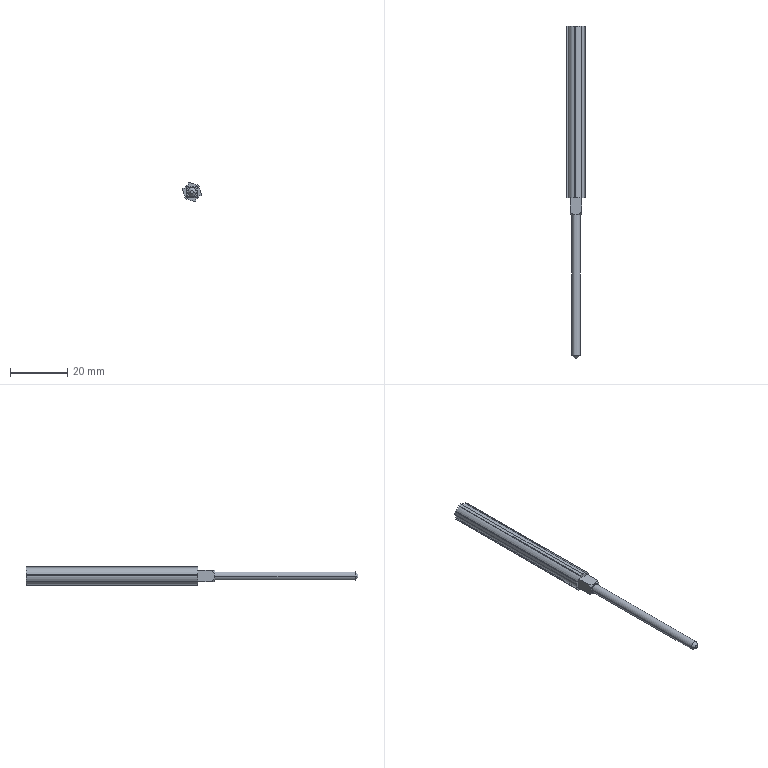Part | STEP file | ASND-0110-Screw gunpart1 | 1 solid | 39 faces | box 6.827 x 116 x 6.827 mm | volume 2290 mm3 | plane 26 | cylinder 9 | cone 4 | commonest cylinder face diameters 6 x7 3 x2